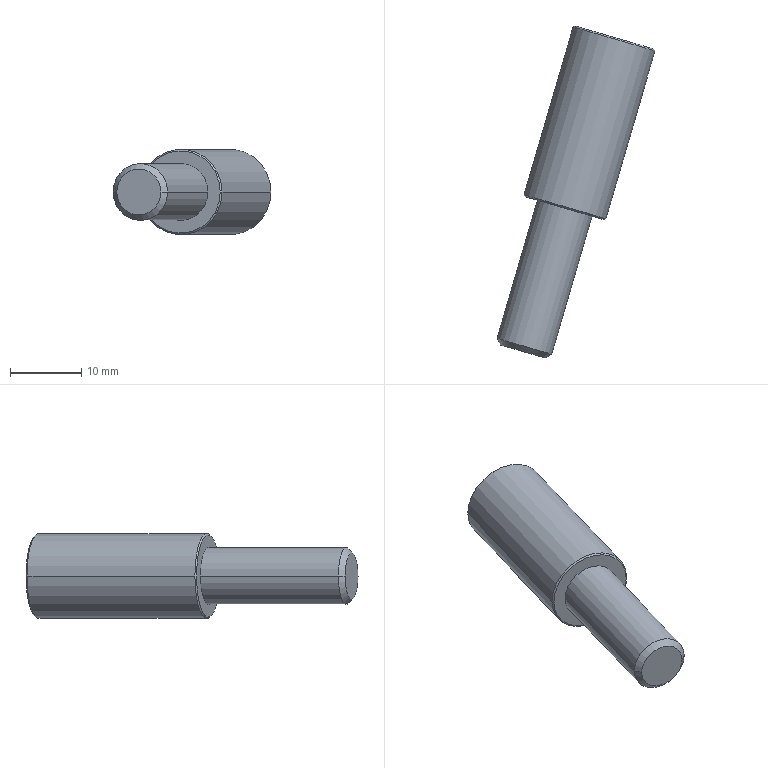Part | SolidWorks | features BaseBody 1 | 1 solid | 31 faces | box 22.207 x 46.689 x 12 mm | volume 3091 mm3 | plane 15 | cone 10 | cylinder 6 | commonest cylinder face diameters 6.647 x2 8 x2 12 x2
STEP:
#1=CARTESIAN_POINT('',(21.689,446.862,-1.629));
#2=VERTEX_POINT('',#1);
#3=CARTESIAN_POINT('',(10.169,450.221,-1.629));
#4=VERTEX_POINT('',#3);
#5=CARTESIAN_POINT('',(15.929,448.541,-1.629));
#6=DIRECTION('',(-0.28,-0.96,0.));
#7=DIRECTION('',(0.96,-0.28,0.));
#8=AXIS2_PLACEMENT_3D('',#5,#6,#7);
#9=CIRCLE('',#8,6.);
#10=EDGE_CURVE('',#2,#4,#9,.T.);
#11=ORIENTED_EDGE('',*,*,#10,.T.);
#12=CARTESIAN_POINT('',(3.282,426.605,-1.629));
#13=VERTEX_POINT('',#12);
#14=CARTESIAN_POINT('',(6.726,438.413,-1.629));
#15=DIRECTION('',(-0.28,-0.96,0.));
#16=VECTOR('',#15,1000.);
#17=LINE('',#14,#16);
#18=EDGE_CURVE('',#4,#13,#17,.T.);
#19=ORIENTED_EDGE('',*,*,#18,.T.);
#20=CARTESIAN_POINT('',(14.802,423.245,-1.629));
#21=VERTEX_POINT('',#20);
#22=CARTESIAN_POINT('',(9.042,424.925,-1.629));
#23=DIRECTION('',(0.28,0.96,0.));
#24=DIRECTION('',(0.96,-0.28,0.));
#25=AXIS2_PLACEMENT_3D('',#22,#23,#24);
#26=CIRCLE('',#25,6.);
#27=EDGE_CURVE('',#13,#21,#26,.T.);
#28=ORIENTED_EDGE('',*,*,#27,.T.);
#29=CARTESIAN_POINT('',(18.246,435.053,-1.629));
#30=DIRECTION('',(-0.28,-0.96,0.));
#31=VECTOR('',#30,1000.);
#32=LINE('',#29,#31);
#33=EDGE_CURVE('',#2,#21,#32,.T.);
#34=ORIENTED_EDGE('',*,*,#33,.F.);
#35=EDGE_LOOP('',(#11,#19,#28,#34));
#36=FACE_OUTER_BOUND('',#35,.T.);
#37=CARTESIAN_POINT('',(12.486,436.733,-1.629));
#38=DIRECTION('',(-0.28,-0.96,0.));
#39=DIRECTION('',(0.96,-0.28,0.));
#40=AXIS2_PLACEMENT_3D('',#37,#38,#39);
#41=CYLINDRICAL_SURFACE('',#40,6.);
#42=ADVANCED_FACE('',(#36),#41,.T.);
#43=CARTESIAN_POINT('',(3.418,426.357,-1.629));
#44=VERTEX_POINT('',#43);
#45=CARTESIAN_POINT('',(14.554,423.109,-1.629));
#46=VERTEX_POINT('',#45);
#47=CARTESIAN_POINT('',(8.986,424.733,-1.629));
#48=DIRECTION('',(0.28,0.96,0.));
#49=DIRECTION('',(-0.96,0.28,0.));
#50=AXIS2_PLACEMENT_3D('',#47,#48,#49);
#51=CIRCLE('',#50,5.8);
#52=EDGE_CURVE('',#44,#46,#51,.T.);
#53=ORIENTED_EDGE('',*,*,#52,.T.);
#54=CARTESIAN_POINT('',(14.802,423.245,-1.629));
#55=DIRECTION('',(0.8768,0.4809,0.));
#56=VECTOR('',#55,1000.);
#57=LINE('',#54,#56);
#58=EDGE_CURVE('',#46,#21,#57,.T.);
#59=ORIENTED_EDGE('',*,*,#58,.T.);
#60=ORIENTED_EDGE('',*,*,#27,.F.);
#61=CARTESIAN_POINT('',(3.282,426.605,-1.629));
#62=DIRECTION('',(-0.4809,0.8768,0.));
#63=VECTOR('',#62,1000.);
#64=LINE('',#61,#63);
#65=EDGE_CURVE('',#44,#13,#64,.T.);
#66=ORIENTED_EDGE('',*,*,#65,.F.);
#67=EDGE_LOOP('',(#53,#59,#60,#66));
#68=FACE_OUTER_BOUND('',#67,.T.);
#69=CARTESIAN_POINT('',(9.042,424.925,-1.629));
#70=DIRECTION('',(0.28,0.96,0.));
#71=DIRECTION('',(-0.96,0.28,0.));
#72=AXIS2_PLACEMENT_3D('',#69,#70,#71);
#73=CONICAL_SURFACE('',#72,6.,0.7854);
#74=ADVANCED_FACE('',(#68),#73,.T.);
#75=CARTESIAN_POINT('',(21.553,447.11,-1.629));
#76=VERTEX_POINT('',#75);
#77=CARTESIAN_POINT('',(10.417,450.357,-1.629));
#78=VERTEX_POINT('',#77);
#79=CARTESIAN_POINT('',(15.985,448.733,-1.629));
#80=DIRECTION('',(-0.28,-0.96,0.));
#81=DIRECTION('',(0.96,-0.28,0.));
#82=AXIS2_PLACEMENT_3D('',#79,#80,#81);
#83=CIRCLE('',#82,5.8);
#84=EDGE_CURVE('',#76,#78,#83,.T.);
#85=ORIENTED_EDGE('',*,*,#84,.T.);
#86=CARTESIAN_POINT('',(10.169,450.221,-1.629));
#87=DIRECTION('',(-0.8768,-0.4809,0.));
#88=VECTOR('',#87,1000.);
#89=LINE('',#86,#88);
#90=EDGE_CURVE('',#78,#4,#89,.T.);
#91=ORIENTED_EDGE('',*,*,#90,.T.);
#92=ORIENTED_EDGE('',*,*,#10,.F.);
#93=CARTESIAN_POINT('',(21.689,446.862,-1.629));
#94=DIRECTION('',(0.4809,-0.8768,0.));
#95=VECTOR('',#94,1000.);
#96=LINE('',#93,#95);
#97=EDGE_CURVE('',#76,#2,#96,.T.);
#98=ORIENTED_EDGE('',*,*,#97,.F.);
#99=EDGE_LOOP('',(#85,#91,#92,#98));
#100=FACE_OUTER_BOUND('',#99,.T.);
#101=CARTESIAN_POINT('',(15.929,448.541,-1.629));
#102=DIRECTION('',(-0.28,-0.96,0.));
#103=DIRECTION('',(0.96,-0.28,0.));
#104=AXIS2_PLACEMENT_3D('',#101,#102,#103);
#105=CONICAL_SURFACE('',#104,6.,0.7854);
#106=ADVANCED_FACE('',(#100),#105,.T.);
#107=CARTESIAN_POINT('',(5.146,425.853,-1.629));
#108=VERTEX_POINT('',#107);
#109=CARTESIAN_POINT('',(12.826,423.613,-1.629));
#110=VERTEX_POINT('',#109);
#111=CARTESIAN_POINT('',(8.986,424.733,-1.629));
#112=DIRECTION('',(0.28,0.96,0.));
#113=DIRECTION('',(0.96,-0.28,0.));
#114=AXIS2_PLACEMENT_3D('',#111,#112,#113);
#115=CIRCLE('',#114,4.);
#116=EDGE_CURVE('',#108,#110,#115,.T.);
#117=ORIENTED_EDGE('',*,*,#116,.F.);
#118=CARTESIAN_POINT('',(-0.5181,406.429,-1.629));
#119=VERTEX_POINT('',#118);
#120=CARTESIAN_POINT('',(2.314,416.141,-1.629));
#121=DIRECTION('',(-0.28,-0.96,0.));
#122=VECTOR('',#121,1000.);
#123=LINE('',#120,#122);
#124=EDGE_CURVE('',#108,#119,#123,.T.);
#125=ORIENTED_EDGE('',*,*,#124,.T.);
#126=CARTESIAN_POINT('',(7.162,404.189,-1.629));
#127=VERTEX_POINT('',#126);
#128=CARTESIAN_POINT('',(3.322,405.309,-1.629));
#129=DIRECTION('',(0.28,0.96,0.));
#130=DIRECTION('',(0.96,-0.28,0.));
#131=AXIS2_PLACEMENT_3D('',#128,#129,#130);
#132=CIRCLE('',#131,4.);
#133=EDGE_CURVE('',#119,#127,#132,.T.);
#134=ORIENTED_EDGE('',*,*,#133,.T.);
#135=CARTESIAN_POINT('',(9.994,413.901,-1.629));
#136=DIRECTION('',(-0.28,-0.96,0.));
#137=VECTOR('',#136,1000.);
#138=LINE('',#135,#137);
#139=EDGE_CURVE('',#110,#127,#138,.T.);
#140=ORIENTED_EDGE('',*,*,#139,.F.);
#141=EDGE_LOOP('',(#117,#125,#134,#140));
#142=FACE_OUTER_BOUND('',#141,.T.);
#143=CARTESIAN_POINT('',(6.154,415.021,-1.629));
#144=DIRECTION('',(-0.28,-0.96,0.));
#145=DIRECTION('',(0.96,-0.28,0.));
#146=AXIS2_PLACEMENT_3D('',#143,#144,#145);
#147=CYLINDRICAL_SURFACE('',#146,4.);
#148=ADVANCED_FACE('',(#142),#147,.T.);
#149=CARTESIAN_POINT('',(0.003527,405.478,-1.629));
#150=VERTEX_POINT('',#149);
#151=CARTESIAN_POINT('',(6.211,403.668,-1.629));
#152=VERTEX_POINT('',#151);
#153=CARTESIAN_POINT('',(3.107,404.573,-1.629));
#154=DIRECTION('',(0.28,0.96,0.));
#155=DIRECTION('',(-0.96,0.28,0.));
#156=AXIS2_PLACEMENT_3D('',#153,#154,#155);
#157=CIRCLE('',#156,3.233);
#158=EDGE_CURVE('',#150,#152,#157,.T.);
#159=ORIENTED_EDGE('',*,*,#158,.T.);
#160=CARTESIAN_POINT('',(7.162,404.189,-1.629));
#161=DIRECTION('',(0.8768,0.4809,0.));
#162=VECTOR('',#161,1000.);
#163=LINE('',#160,#162);
#164=EDGE_CURVE('',#152,#127,#163,.T.);
#165=ORIENTED_EDGE('',*,*,#164,.T.);
#166=ORIENTED_EDGE('',*,*,#133,.F.);
#167=CARTESIAN_POINT('',(-0.5181,406.429,-1.629));
#168=DIRECTION('',(-0.4809,0.8768,0.));
#169=VECTOR('',#168,1000.);
#170=LINE('',#167,#169);
#171=EDGE_CURVE('',#150,#119,#170,.T.);
#172=ORIENTED_EDGE('',*,*,#171,.F.);
#173=EDGE_LOOP('',(#159,#165,#166,#172));
#174=FACE_OUTER_BOUND('',#173,.T.);
#175=CARTESIAN_POINT('',(3.322,405.309,-1.629));
#176=DIRECTION('',(0.28,0.96,0.));
#177=DIRECTION('',(-0.96,0.28,0.));
#178=AXIS2_PLACEMENT_3D('',#175,#176,#177);
#179=CONICAL_SURFACE('',#178,4.,0.7854);
#180=ADVANCED_FACE('',(#174),#179,.T.);
#181=CARTESIAN_POINT('',(18.146,444.273,-1.629));
#182=VERTEX_POINT('',#181);
#183=CARTESIAN_POINT('',(11.765,446.134,-1.629));
#184=VERTEX_POINT('',#183);
#185=CARTESIAN_POINT('',(14.956,445.204,-1.629));
#186=DIRECTION('',(0.28,0.96,0.));
#187=DIRECTION('',(0.,0.,1.));
#188=AXIS2_PLACEMENT_3D('',#185,#186,#187);
#189=CIRCLE('',#188,3.324);
#190=EDGE_CURVE('',#182,#184,#189,.T.);
#191=ORIENTED_EDGE('',*,*,#190,.F.);
#192=CARTESIAN_POINT('',(18.985,444.733,-1.629));
#193=VERTEX_POINT('',#192);
#194=CARTESIAN_POINT('',(18.985,444.733,-1.629));
#195=DIRECTION('',(0.8768,0.4809,0.));
#196=VECTOR('',#195,1000.);
#197=LINE('',#194,#196);
#198=EDGE_CURVE('',#182,#193,#197,.T.);
#199=ORIENTED_EDGE('',*,*,#198,.T.);
#200=CARTESIAN_POINT('',(17.065,445.293,-5.093));
#201=VERTEX_POINT('',#200);
#202=CARTESIAN_POINT('',(15.145,445.853,-1.629));
#203=DIRECTION('',(0.28,0.96,0.));
#204=DIRECTION('',(-0.96,0.28,0.));
#205=AXIS2_PLACEMENT_3D('',#202,#203,#204);
#206=CIRCLE('',#205,4.);
#207=EDGE_CURVE('',#193,#201,#206,.T.);
#208=ORIENTED_EDGE('',*,*,#207,.T.);
#209=CARTESIAN_POINT('',(13.225,446.413,-5.093));
#210=VERTEX_POINT('',#209);
#211=CARTESIAN_POINT('',(15.145,445.853,-1.629));
#212=DIRECTION('',(0.28,0.96,0.));
#213=DIRECTION('',(-0.96,0.28,0.));
#214=AXIS2_PLACEMENT_3D('',#211,#212,#213);
#215=CIRCLE('',#214,4.);
#216=EDGE_CURVE('',#201,#210,#215,.T.);
#217=ORIENTED_EDGE('',*,*,#216,.T.);
#218=CARTESIAN_POINT('',(11.305,446.973,-1.629));
#219=VERTEX_POINT('',#218);
#220=CARTESIAN_POINT('',(15.145,445.853,-1.629));
#221=DIRECTION('',(0.28,0.96,0.));
#222=DIRECTION('',(-0.96,0.28,0.));
#223=AXIS2_PLACEMENT_3D('',#220,#221,#222);
#224=CIRCLE('',#223,4.);
#225=EDGE_CURVE('',#210,#219,#224,.T.);
#226=ORIENTED_EDGE('',*,*,#225,.T.);
#227=CARTESIAN_POINT('',(11.305,446.973,-1.629));
#228=DIRECTION('',(-0.4809,0.8768,0.));
#229=VECTOR('',#228,1000.);
#230=LINE('',#227,#229);
#231=EDGE_CURVE('',#184,#219,#230,.T.);
#232=ORIENTED_EDGE('',*,*,#231,.F.);
#233=EDGE_LOOP('',(#191,#199,#208,#217,#226,#232));
#234=FACE_OUTER_BOUND('',#233,.T.);
#235=CARTESIAN_POINT('',(15.145,445.853,-1.629));
#236=DIRECTION('',(0.28,0.96,0.));
#237=DIRECTION('',(-0.96,0.28,0.));
#238=AXIS2_PLACEMENT_3D('',#235,#236,#237);
#239=CONICAL_SURFACE('',#238,4.,0.7854);
#240=ADVANCED_FACE('',(#234),#239,.F.);
#241=ORIENTED_EDGE('',*,*,#190,.T.);
#242=CARTESIAN_POINT('',(7.195,430.463,-1.629));
#243=VERTEX_POINT('',#242);
#244=CARTESIAN_POINT('',(9.48,438.299,-1.629));
#245=DIRECTION('',(-0.28,-0.96,0.));
#246=VECTOR('',#245,1000.);
#247=LINE('',#244,#246);
#248=EDGE_CURVE('',#184,#243,#247,.T.);
#249=ORIENTED_EDGE('',*,*,#248,.T.);
#250=CARTESIAN_POINT('',(13.577,428.603,-1.629));
#251=VERTEX_POINT('',#250);
#252=CARTESIAN_POINT('',(10.386,429.533,-1.629));
#253=DIRECTION('',(0.28,0.96,0.));
#254=DIRECTION('',(0.96,-0.28,0.));
#255=AXIS2_PLACEMENT_3D('',#252,#253,#254);
#256=CIRCLE('',#255,3.324);
#257=EDGE_CURVE('',#251,#243,#256,.T.);
#258=ORIENTED_EDGE('',*,*,#257,.F.);
#259=CARTESIAN_POINT('',(15.862,436.438,-1.629));
#260=DIRECTION('',(-0.28,-0.96,0.));
#261=VECTOR('',#260,1000.);
#262=LINE('',#259,#261);
#263=EDGE_CURVE('',#182,#251,#262,.T.);
#264=ORIENTED_EDGE('',*,*,#263,.F.);
#265=EDGE_LOOP('',(#241,#249,#258,#264));
#266=FACE_OUTER_BOUND('',#265,.T.);
#267=CARTESIAN_POINT('',(12.671,437.368,-1.629));
#268=DIRECTION('',(-0.28,-0.96,0.));
#269=DIRECTION('',(0.96,-0.28,0.));
#270=AXIS2_PLACEMENT_3D('',#267,#268,#269);
#271=CYLINDRICAL_SURFACE('',#270,3.324);
#272=ADVANCED_FACE('',(#266),#271,.F.);
#273=CARTESIAN_POINT('',(9.849,427.691,-1.629));
#274=VERTEX_POINT('',#273);
#275=CARTESIAN_POINT('',(7.195,430.463,-1.629));
#276=DIRECTION('',(-0.6914,0.7225,0.));
#277=VECTOR('',#276,1000.);
#278=LINE('',#275,#277);
#279=EDGE_CURVE('',#274,#243,#278,.T.);
#280=ORIENTED_EDGE('',*,*,#279,.F.);
#281=CARTESIAN_POINT('',(13.577,428.603,-1.629));
#282=DIRECTION('',(0.9714,0.2376,0.));
#283=VECTOR('',#282,1000.);
#284=LINE('',#281,#283);
#285=EDGE_CURVE('',#274,#251,#284,.T.);
#286=ORIENTED_EDGE('',*,*,#285,.T.);
#287=ORIENTED_EDGE('',*,*,#257,.T.);
#288=EDGE_LOOP('',(#280,#286,#287));
#289=FACE_OUTER_BOUND('',#288,.T.);
#290=CARTESIAN_POINT('',(10.386,429.533,-1.629));
#291=DIRECTION('',(0.28,0.96,0.));
#292=DIRECTION('',(-0.96,0.28,0.));
#293=AXIS2_PLACEMENT_3D('',#290,#291,#292);
#294=CONICAL_SURFACE('',#293,3.324,1.047);
#295=ADVANCED_FACE('',(#289),#294,.F.);
#296=ORIENTED_EDGE('',*,*,#18,.F.);
#297=CARTESIAN_POINT('',(15.929,448.541,-1.629));
#298=DIRECTION('',(-0.28,-0.96,0.));
#299=DIRECTION('',(0.96,-0.28,0.));
#300=AXIS2_PLACEMENT_3D('',#297,#298,#299);
#301=CIRCLE('',#300,6.);
#302=EDGE_CURVE('',#4,#2,#301,.T.);
#303=ORIENTED_EDGE('',*,*,#302,.T.);
#304=ORIENTED_EDGE('',*,*,#33,.T.);
#305=CARTESIAN_POINT('',(9.042,424.925,-1.629));
#306=DIRECTION('',(0.28,0.96,0.));
#307=DIRECTION('',(0.96,-0.28,0.));
#308=AXIS2_PLACEMENT_3D('',#305,#306,#307);
#309=CIRCLE('',#308,6.);
#310=EDGE_CURVE('',#21,#13,#309,.T.);
#311=ORIENTED_EDGE('',*,*,#310,.T.);
#312=EDGE_LOOP('',(#296,#303,#304,#311));
#313=FACE_OUTER_BOUND('',#312,.T.);
#314=CARTESIAN_POINT('',(12.486,436.733,-1.629));
#315=DIRECTION('',(-0.28,-0.96,0.));
#316=DIRECTION('',(0.96,-0.28,0.));
#317=AXIS2_PLACEMENT_3D('',#314,#315,#316);
#318=CYLINDRICAL_SURFACE('',#317,6.);
#319=ADVANCED_FACE('',(#313),#318,.T.);
#320=ORIENTED_EDGE('',*,*,#58,.F.);
#321=CARTESIAN_POINT('',(8.986,424.733,-1.629));
#322=DIRECTION('',(0.28,0.96,0.));
#323=DIRECTION('',(-0.96,0.28,0.));
#324=AXIS2_PLACEMENT_3D('',#321,#322,#323);
#325=CIRCLE('',#324,5.8);
#326=EDGE_CURVE('',#46,#44,#325,.T.);
#327=ORIENTED_EDGE('',*,*,#326,.T.);
#328=ORIENTED_EDGE('',*,*,#65,.T.);
#329=ORIENTED_EDGE('',*,*,#310,.F.);
#330=EDGE_LOOP('',(#320,#327,#328,#329));
#331=FACE_OUTER_BOUND('',#330,.T.);
#332=CARTESIAN_POINT('',(9.042,424.925,-1.629));
#333=DIRECTION('',(0.28,0.96,0.));
#334=DIRECTION('',(-0.96,0.28,0.));
#335=AXIS2_PLACEMENT_3D('',#332,#333,#334);
#336=CONICAL_SURFACE('',#335,6.,0.7854);
#337=ADVANCED_FACE('',(#331),#336,.T.);
#338=ORIENTED_EDGE('',*,*,#90,.F.);
#339=CARTESIAN_POINT('',(15.985,448.733,-1.629));
#340=DIRECTION('',(-0.28,-0.96,0.));
#341=DIRECTION('',(0.96,-0.28,0.));
#342=AXIS2_PLACEMENT_3D('',#339,#340,#341);
#343=CIRCLE('',#342,5.8);
#344=EDGE_CURVE('',#78,#76,#343,.T.);
#345=ORIENTED_EDGE('',*,*,#344,.T.);
#346=ORIENTED_EDGE('',*,*,#97,.T.);
#347=ORIENTED_EDGE('',*,*,#302,.F.);
#348=EDGE_LOOP('',(#338,#345,#346,#347));
#349=FACE_OUTER_BOUND('',#348,.T.);
#350=CARTESIAN_POINT('',(15.929,448.541,-1.629));
#351=DIRECTION('',(-0.28,-0.96,0.));
#352=DIRECTION('',(0.96,-0.28,0.));
#353=AXIS2_PLACEMENT_3D('',#350,#351,#352);
#354=CONICAL_SURFACE('',#353,6.,0.7854);
#355=ADVANCED_FACE('',(#349),#354,.T.);
#356=ORIENTED_EDGE('',*,*,#52,.F.);
#357=ORIENTED_EDGE('',*,*,#326,.F.);
#358=EDGE_LOOP('',(#356,#357));
#359=FACE_OUTER_BOUND('',#358,.T.);
#360=CARTESIAN_POINT('',(8.986,424.733,-1.629));
#361=DIRECTION('',(0.28,0.96,0.));
#362=DIRECTION('',(0.96,-0.28,0.));
#363=AXIS2_PLACEMENT_3D('',#360,#361,#362);
#364=CIRCLE('',#363,4.);
#365=EDGE_CURVE('',#110,#108,#364,.T.);
#366=ORIENTED_EDGE('',*,*,#365,.T.);
#367=ORIENTED_EDGE('',*,*,#116,.T.);
#368=EDGE_LOOP('',(#366,#367));
#369=FACE_BOUND('',#368,.T.);
#370=CARTESIAN_POINT('',(8.986,424.733,1.271));
#371=DIRECTION('',(-0.28,-0.96,0.));
#372=DIRECTION('',(0.96,-0.28,0.));
#373=AXIS2_PLACEMENT_3D('',#370,#371,#372);
#374=PLANE('',#373);
#375=ADVANCED_FACE('',(#359,#369),#374,.T.);
#376=CARTESIAN_POINT('',(12.145,449.853,-3.938));
#377=VERTEX_POINT('',#376);
#378=CARTESIAN_POINT('',(15.985,448.733,-6.248));
#379=VERTEX_POINT('',#378);
#380=CARTESIAN_POINT('',(12.145,449.853,-3.938));
#381=DIRECTION('',(0.8314,-0.2424,-0.5));
#382=VECTOR('',#381,1000.);
#383=LINE('',#380,#382);
#384=EDGE_CURVE('',#377,#379,#383,.T.);
#385=ORIENTED_EDGE('',*,*,#384,.T.);
#386=CARTESIAN_POINT('',(19.825,447.613,-3.938));
#387=VERTEX_POINT('',#386);
#388=CARTESIAN_POINT('',(15.985,448.733,-6.248));
#389=DIRECTION('',(0.8314,-0.2424,0.5));
#390=VECTOR('',#389,1000.);
#391=LINE('',#388,#390);
#392=EDGE_CURVE('',#379,#387,#391,.T.);
#393=ORIENTED_EDGE('',*,*,#392,.T.);
#394=CARTESIAN_POINT('',(19.825,447.613,0.6805));
#395=VERTEX_POINT('',#394);
#396=CARTESIAN_POINT('',(19.825,447.613,1.271));
#397=DIRECTION('',(0.,0.,1.));
#398=VECTOR('',#397,1000.);
#399=LINE('',#396,#398);
#400=EDGE_CURVE('',#387,#395,#399,.T.);
#401=ORIENTED_EDGE('',*,*,#400,.T.);
#402=CARTESIAN_POINT('',(15.985,448.733,2.99));
#403=VERTEX_POINT('',#402);
#404=CARTESIAN_POINT('',(19.825,447.613,0.6805));
#405=DIRECTION('',(-0.8314,0.2424,0.5));
#406=VECTOR('',#405,1000.);
#407=LINE('',#404,#406);
#408=EDGE_CURVE('',#395,#403,#407,.T.);
#409=ORIENTED_EDGE('',*,*,#408,.T.);
#410=CARTESIAN_POINT('',(12.145,449.853,0.6805));
#411=VERTEX_POINT('',#410);
#412=CARTESIAN_POINT('',(15.985,448.733,2.99));
#413=DIRECTION('',(-0.8314,0.2424,-0.5));
#414=VECTOR('',#413,1000.);
#415=LINE('',#412,#414);
#416=EDGE_CURVE('',#403,#411,#415,.T.);
#417=ORIENTED_EDGE('',*,*,#416,.T.);
#418=CARTESIAN_POINT('',(12.145,449.853,1.271));
#419=DIRECTION('',(0.,0.,-1.));
#420=VECTOR('',#419,1000.);
#421=LINE('',#418,#420);
#422=EDGE_CURVE('',#411,#377,#421,.T.);
#423=ORIENTED_EDGE('',*,*,#422,.T.);
#424=EDGE_LOOP('',(#385,#393,#401,#409,#417,#423));
#425=FACE_BOUND('',#424,.T.);
#426=ORIENTED_EDGE('',*,*,#84,.F.);
#427=ORIENTED_EDGE('',*,*,#344,.F.);
#428=EDGE_LOOP('',(#426,#427));
#429=FACE_OUTER_BOUND('',#428,.T.);
#430=CARTESIAN_POINT('',(15.985,448.733,1.271));
#431=DIRECTION('',(0.28,0.96,0.));
#432=DIRECTION('',(-0.96,0.28,0.));
#433=AXIS2_PLACEMENT_3D('',#430,#431,#432);
#434=PLANE('',#433);
#435=ADVANCED_FACE('',(#425,#429),#434,.T.);
#436=ORIENTED_EDGE('',*,*,#124,.F.);
#437=ORIENTED_EDGE('',*,*,#365,.F.);
#438=ORIENTED_EDGE('',*,*,#139,.T.);
#439=CARTESIAN_POINT('',(3.322,405.309,-1.629));
#440=DIRECTION('',(0.28,0.96,0.));
#441=DIRECTION('',(0.96,-0.28,0.));
#442=AXIS2_PLACEMENT_3D('',#439,#440,#441);
#443=CIRCLE('',#442,4.);
#444=EDGE_CURVE('',#127,#119,#443,.T.);
#445=ORIENTED_EDGE('',*,*,#444,.T.);
#446=EDGE_LOOP('',(#436,#437,#438,#445));
#447=FACE_OUTER_BOUND('',#446,.T.);
#448=CARTESIAN_POINT('',(6.154,415.021,-1.629));
#449=DIRECTION('',(-0.28,-0.96,0.));
#450=DIRECTION('',(0.96,-0.28,0.));
#451=AXIS2_PLACEMENT_3D('',#448,#449,#450);
#452=CYLINDRICAL_SURFACE('',#451,4.);
#453=ADVANCED_FACE('',(#447),#452,.T.);
#454=ORIENTED_EDGE('',*,*,#392,.F.);
#455=CARTESIAN_POINT('',(15.145,445.853,-6.248));
#456=VERTEX_POINT('',#455);
#457=CARTESIAN_POINT('',(15.145,445.853,-6.248));
#458=DIRECTION('',(0.28,0.96,0.));
#459=VECTOR('',#458,1000.);
#460=LINE('',#457,#459);
#461=EDGE_CURVE('',#456,#379,#460,.T.);
#462=ORIENTED_EDGE('',*,*,#461,.F.);
#463=CARTESIAN_POINT('',(17.065,445.293,-5.093));
#464=DIRECTION('',(-0.8314,0.2424,-0.5));
#465=VECTOR('',#464,1000.);
#466=LINE('',#463,#465);
#467=EDGE_CURVE('',#201,#456,#466,.T.);
#468=ORIENTED_EDGE('',*,*,#467,.F.);
#469=CARTESIAN_POINT('',(18.985,444.733,-3.938));
#470=VERTEX_POINT('',#469);
#471=CARTESIAN_POINT('',(18.985,444.733,-3.938));
#472=DIRECTION('',(-0.8314,0.2424,-0.5));
#473=VECTOR('',#472,1000.);
#474=LINE('',#471,#473);
#475=EDGE_CURVE('',#470,#201,#474,.T.);
#476=ORIENTED_EDGE('',*,*,#475,.F.);
#477=CARTESIAN_POINT('',(19.825,447.613,-3.938));
#478=DIRECTION('',(-0.28,-0.96,0.));
#479=VECTOR('',#478,1000.);
#480=LINE('',#477,#479);
#481=EDGE_CURVE('',#387,#470,#480,.T.);
#482=ORIENTED_EDGE('',*,*,#481,.F.);
#483=EDGE_LOOP('',(#454,#462,#468,#476,#482));
#484=FACE_OUTER_BOUND('',#483,.T.);
#485=CARTESIAN_POINT('',(19.825,447.613,-3.938));
#486=DIRECTION('',(0.48,-0.14,-0.866));
#487=DIRECTION('',(-0.8746,0.,-0.4848));
#488=AXIS2_PLACEMENT_3D('',#485,#486,#487);
#489=PLANE('',#488);
#490=ADVANCED_FACE('',(#484),#489,.F.);
#491=ORIENTED_EDGE('',*,*,#384,.F.);
#492=CARTESIAN_POINT('',(11.305,446.973,-3.938));
#493=VERTEX_POINT('',#492);
#494=CARTESIAN_POINT('',(11.305,446.973,-3.938));
#495=DIRECTION('',(0.28,0.96,0.));
#496=VECTOR('',#495,1000.);
#497=LINE('',#494,#496);
#498=EDGE_CURVE('',#493,#377,#497,.T.);
#499=ORIENTED_EDGE('',*,*,#498,.F.);
#500=CARTESIAN_POINT('',(13.225,446.413,-5.093));
#501=DIRECTION('',(-0.8314,0.2424,0.5));
#502=VECTOR('',#501,1000.);
#503=LINE('',#500,#502);
#504=EDGE_CURVE('',#210,#493,#503,.T.);
#505=ORIENTED_EDGE('',*,*,#504,.F.);
#506=CARTESIAN_POINT('',(15.145,445.853,-6.248));
#507=DIRECTION('',(-0.8314,0.2424,0.5));
#508=VECTOR('',#507,1000.);
#509=LINE('',#506,#508);
#510=EDGE_CURVE('',#456,#210,#509,.T.);
#511=ORIENTED_EDGE('',*,*,#510,.F.);
#512=ORIENTED_EDGE('',*,*,#461,.T.);
#513=EDGE_LOOP('',(#491,#499,#505,#511,#512));
#514=FACE_OUTER_BOUND('',#513,.T.);
#515=CARTESIAN_POINT('',(15.985,448.733,-6.248));
#516=DIRECTION('',(-0.48,0.14,-0.866));
#517=DIRECTION('',(-0.8746,0.,0.4848));
#518=AXIS2_PLACEMENT_3D('',#515,#516,#517);
#519=PLANE('',#518);
#520=ADVANCED_FACE('',(#514),#519,.F.);
#521=ORIENTED_EDGE('',*,*,#422,.F.);
#522=CARTESIAN_POINT('',(11.305,446.973,0.6805));
#523=VERTEX_POINT('',#522);
#524=CARTESIAN_POINT('',(12.145,449.853,0.6805));
#525=DIRECTION('',(0.28,0.96,0.));
#526=VECTOR('',#525,1000.);
#527=LINE('',#524,#526);
#528=EDGE_CURVE('',#523,#411,#527,.T.);
#529=ORIENTED_EDGE('',*,*,#528,.F.);
#530=CARTESIAN_POINT('',(11.305,446.973,-3.938));
#531=DIRECTION('',(0.,0.,1.));
#532=VECTOR('',#531,1000.);
#533=LINE('',#530,#532);
#534=EDGE_CURVE('',#219,#523,#533,.T.);
#535=ORIENTED_EDGE('',*,*,#534,.F.);
#536=CARTESIAN_POINT('',(11.305,446.973,-3.938));
#537=DIRECTION('',(0.,0.,1.));
#538=VECTOR('',#537,1000.);
#539=LINE('',#536,#538);
#540=EDGE_CURVE('',#493,#219,#539,.T.);
#541=ORIENTED_EDGE('',*,*,#540,.F.);
#542=ORIENTED_EDGE('',*,*,#498,.T.);
#543=EDGE_LOOP('',(#521,#529,#535,#541,#542));
#544=FACE_OUTER_BOUND('',#543,.T.);
#545=CARTESIAN_POINT('',(12.145,449.853,-3.938));
#546=DIRECTION('',(-0.96,0.28,0.));
#547=DIRECTION('',(-0.28,-0.96,0.));
#548=AXIS2_PLACEMENT_3D('',#545,#546,#547);
#549=PLANE('',#548);
#550=ADVANCED_FACE('',(#544),#549,.F.);
#551=ORIENTED_EDGE('',*,*,#416,.F.);
#552=CARTESIAN_POINT('',(15.145,445.853,2.99));
#553=VERTEX_POINT('',#552);
#554=CARTESIAN_POINT('',(15.145,445.853,2.99));
#555=DIRECTION('',(0.28,0.96,0.));
#556=VECTOR('',#555,1000.);
#557=LINE('',#554,#556);
#558=EDGE_CURVE('',#553,#403,#557,.T.);
#559=ORIENTED_EDGE('',*,*,#558,.F.);
#560=CARTESIAN_POINT('',(13.225,446.413,1.835));
#561=VERTEX_POINT('',#560);
#562=CARTESIAN_POINT('',(13.225,446.413,1.835));
#563=DIRECTION('',(0.8314,-0.2424,0.5));
#564=VECTOR('',#563,1000.);
#565=LINE('',#562,#564);
#566=EDGE_CURVE('',#561,#553,#565,.T.);
#567=ORIENTED_EDGE('',*,*,#566,.F.);
#568=CARTESIAN_POINT('',(11.305,446.973,0.6805));
#569=DIRECTION('',(0.8314,-0.2424,0.5));
#570=VECTOR('',#569,1000.);
#571=LINE('',#568,#570);
#572=EDGE_CURVE('',#523,#561,#571,.T.);
#573=ORIENTED_EDGE('',*,*,#572,.F.);
#574=ORIENTED_EDGE('',*,*,#528,.T.);
#575=EDGE_LOOP('',(#551,#559,#567,#573,#574));
#576=FACE_OUTER_BOUND('',#575,.T.);
#577=CARTESIAN_POINT('',(12.145,449.853,0.6805));
#578=DIRECTION('',(-0.48,0.14,0.866));
#579=DIRECTION('',(0.8746,0.,0.4848));
#580=AXIS2_PLACEMENT_3D('',#577,#578,#579);
#581=PLANE('',#580);
#582=ADVANCED_FACE('',(#576),#581,.F.);
#583=ORIENTED_EDGE('',*,*,#408,.F.);
#584=CARTESIAN_POINT('',(18.985,444.733,0.6805));
#585=VERTEX_POINT('',#584);
#586=CARTESIAN_POINT('',(18.985,444.733,0.6805));
#587=DIRECTION('',(0.28,0.96,0.));
#588=VECTOR('',#587,1000.);
#589=LINE('',#586,#588);
#590=EDGE_CURVE('',#585,#395,#589,.T.);
#591=ORIENTED_EDGE('',*,*,#590,.F.);
#592=CARTESIAN_POINT('',(17.065,445.293,1.835));
#593=VERTEX_POINT('',#592);
#594=CARTESIAN_POINT('',(17.065,445.293,1.835));
#595=DIRECTION('',(0.8314,-0.2424,-0.5));
#596=VECTOR('',#595,1000.);
#597=LINE('',#594,#596);
#598=EDGE_CURVE('',#593,#585,#597,.T.);
#599=ORIENTED_EDGE('',*,*,#598,.F.);
#600=CARTESIAN_POINT('',(15.145,445.853,2.99));
#601=DIRECTION('',(0.8314,-0.2424,-0.5));
#602=VECTOR('',#601,1000.);
#603=LINE('',#600,#602);
#604=EDGE_CURVE('',#553,#593,#603,.T.);
#605=ORIENTED_EDGE('',*,*,#604,.F.);
#606=ORIENTED_EDGE('',*,*,#558,.T.);
#607=EDGE_LOOP('',(#583,#591,#599,#605,#606));
#608=FACE_OUTER_BOUND('',#607,.T.);
#609=CARTESIAN_POINT('',(15.985,448.733,2.99));
#610=DIRECTION('',(0.48,-0.14,0.866));
#611=DIRECTION('',(0.8746,0.,-0.4848));
#612=AXIS2_PLACEMENT_3D('',#609,#610,#611);
#613=PLANE('',#612);
#614=ADVANCED_FACE('',(#608),#613,.F.);
#615=ORIENTED_EDGE('',*,*,#400,.F.);
#616=ORIENTED_EDGE('',*,*,#481,.T.);
#617=CARTESIAN_POINT('',(18.985,444.733,0.6805));
#618=DIRECTION('',(0.,0.,-1.));
#619=VECTOR('',#618,1000.);
#620=LINE('',#617,#619);
#621=EDGE_CURVE('',#193,#470,#620,.T.);
#622=ORIENTED_EDGE('',*,*,#621,.F.);
#623=CARTESIAN_POINT('',(18.985,444.733,0.6805));
#624=DIRECTION('',(0.,0.,-1.));
#625=VECTOR('',#624,1000.);
#626=LINE('',#623,#625);
#627=EDGE_CURVE('',#585,#193,#626,.T.);
#628=ORIENTED_EDGE('',*,*,#627,.F.);
#629=ORIENTED_EDGE('',*,*,#590,.T.);
#630=EDGE_LOOP('',(#615,#616,#622,#628,#629));
#631=FACE_OUTER_BOUND('',#630,.T.);
#632=CARTESIAN_POINT('',(19.825,447.613,0.6805));
#633=DIRECTION('',(0.96,-0.28,0.));
#634=DIRECTION('',(0.28,0.96,0.));
#635=AXIS2_PLACEMENT_3D('',#632,#633,#634);
#636=PLANE('',#635);
#637=ADVANCED_FACE('',(#631),#636,.F.);
#638=ORIENTED_EDGE('',*,*,#164,.F.);
#639=CARTESIAN_POINT('',(3.107,404.573,-1.629));
#640=DIRECTION('',(0.28,0.96,0.));
#641=DIRECTION('',(-0.96,0.28,0.));
#642=AXIS2_PLACEMENT_3D('',#639,#640,#641);
#643=CIRCLE('',#642,3.233);
#644=EDGE_CURVE('',#152,#150,#643,.T.);
#645=ORIENTED_EDGE('',*,*,#644,.T.);
#646=ORIENTED_EDGE('',*,*,#171,.T.);
#647=ORIENTED_EDGE('',*,*,#444,.F.);
#648=EDGE_LOOP('',(#638,#645,#646,#647));
#649=FACE_OUTER_BOUND('',#648,.T.);
#650=CARTESIAN_POINT('',(3.322,405.309,-1.629));
#651=DIRECTION('',(0.28,0.96,0.));
#652=DIRECTION('',(-0.96,0.28,0.));
#653=AXIS2_PLACEMENT_3D('',#650,#651,#652);
#654=CONICAL_SURFACE('',#653,4.,0.7854);
#655=ADVANCED_FACE('',(#649),#654,.T.);
#656=ORIENTED_EDGE('',*,*,#467,.T.);
#657=ORIENTED_EDGE('',*,*,#510,.T.);
#658=ORIENTED_EDGE('',*,*,#216,.F.);
#659=EDGE_LOOP('',(#656,#657,#658));
#660=FACE_OUTER_BOUND('',#659,.T.);
#661=CARTESIAN_POINT('',(15.145,445.853,-1.629));
#662=DIRECTION('',(-0.28,-0.96,0.));
#663=DIRECTION('',(0.96,-0.28,0.));
#664=AXIS2_PLACEMENT_3D('',#661,#662,#663);
#665=PLANE('',#664);
#666=ADVANCED_FACE('',(#660),#665,.F.);
#667=ORIENTED_EDGE('',*,*,#475,.T.);
#668=ORIENTED_EDGE('',*,*,#207,.F.);
#669=ORIENTED_EDGE('',*,*,#621,.T.);
#670=EDGE_LOOP('',(#667,#668,#669));
#671=FACE_OUTER_BOUND('',#670,.T.);
#672=CARTESIAN_POINT('',(15.145,445.853,-1.629));
#673=DIRECTION('',(-0.28,-0.96,0.));
#674=DIRECTION('',(0.96,-0.28,0.));
#675=AXIS2_PLACEMENT_3D('',#672,#673,#674);
#676=PLANE('',#675);
#677=ADVANCED_FACE('',(#671),#676,.F.);
#678=ORIENTED_EDGE('',*,*,#540,.T.);
#679=ORIENTED_EDGE('',*,*,#225,.F.);
#680=ORIENTED_EDGE('',*,*,#504,.T.);
#681=EDGE_LOOP('',(#678,#679,#680));
#682=FACE_OUTER_BOUND('',#681,.T.);
#683=CARTESIAN_POINT('',(15.145,445.853,-1.629));
#684=DIRECTION('',(-0.28,-0.96,0.));
#685=DIRECTION('',(0.96,-0.28,0.));
#686=AXIS2_PLACEMENT_3D('',#683,#684,#685);
#687=PLANE('',#686);
#688=ADVANCED_FACE('',(#682),#687,.F.);
#689=ORIENTED_EDGE('',*,*,#572,.T.);
#690=CARTESIAN_POINT('',(15.145,445.853,-1.629));
#691=DIRECTION('',(0.28,0.96,0.));
#692=DIRECTION('',(-0.96,0.28,0.));
#693=AXIS2_PLACEMENT_3D('',#690,#691,#692);
#694=CIRCLE('',#693,4.);
#695=EDGE_CURVE('',#219,#561,#694,.T.);
#696=ORIENTED_EDGE('',*,*,#695,.F.);
#697=ORIENTED_EDGE('',*,*,#534,.T.);
#698=EDGE_LOOP('',(#689,#696,#697));
#699=FACE_OUTER_BOUND('',#698,.T.);
#700=CARTESIAN_POINT('',(15.145,445.853,-1.629));
#701=DIRECTION('',(-0.28,-0.96,0.));
#702=DIRECTION('',(0.96,-0.28,0.));
#703=AXIS2_PLACEMENT_3D('',#700,#701,#702);
#704=PLANE('',#703);
#705=ADVANCED_FACE('',(#699),#704,.F.);
#706=ORIENTED_EDGE('',*,*,#566,.T.);
#707=ORIENTED_EDGE('',*,*,#604,.T.);
#708=CARTESIAN_POINT('',(15.145,445.853,-1.629));
#709=DIRECTION('',(0.28,0.96,0.));
#710=DIRECTION('',(-0.96,0.28,0.));
#711=AXIS2_PLACEMENT_3D('',#708,#709,#710);
#712=CIRCLE('',#711,4.);
#713=EDGE_CURVE('',#561,#593,#712,.T.);
#714=ORIENTED_EDGE('',*,*,#713,.F.);
#715=EDGE_LOOP('',(#706,#707,#714));
#716=FACE_OUTER_BOUND('',#715,.T.);
#717=CARTESIAN_POINT('',(15.145,445.853,-1.629));
#718=DIRECTION('',(-0.28,-0.96,0.));
#719=DIRECTION('',(0.96,-0.28,0.));
#720=AXIS2_PLACEMENT_3D('',#717,#718,#719);
#721=PLANE('',#720);
#722=ADVANCED_FACE('',(#716),#721,.F.);
#723=ORIENTED_EDGE('',*,*,#627,.T.);
#724=CARTESIAN_POINT('',(15.145,445.853,-1.629));
#725=DIRECTION('',(0.28,0.96,0.));
#726=DIRECTION('',(-0.96,0.28,0.));
#727=AXIS2_PLACEMENT_3D('',#724,#725,#726);
#728=CIRCLE('',#727,4.);
#729=EDGE_CURVE('',#593,#193,#728,.T.);
#730=ORIENTED_EDGE('',*,*,#729,.F.);
#731=ORIENTED_EDGE('',*,*,#598,.T.);
#732=EDGE_LOOP('',(#723,#730,#731));
#733=FACE_OUTER_BOUND('',#732,.T.);
#734=CARTESIAN_POINT('',(15.145,445.853,-1.629));
#735=DIRECTION('',(-0.28,-0.96,0.));
#736=DIRECTION('',(0.96,-0.28,0.));
#737=AXIS2_PLACEMENT_3D('',#734,#735,#736);
#738=PLANE('',#737);
#739=ADVANCED_FACE('',(#733),#738,.F.);
#740=ORIENTED_EDGE('',*,*,#158,.F.);
#741=ORIENTED_EDGE('',*,*,#644,.F.);
#742=EDGE_LOOP('',(#740,#741));
#743=FACE_OUTER_BOUND('',#742,.T.);
#744=CARTESIAN_POINT('',(3.107,404.573,-0.01242));
#745=DIRECTION('',(-0.28,-0.96,0.));
#746=DIRECTION('',(0.96,-0.28,0.));
#747=AXIS2_PLACEMENT_3D('',#744,#745,#746);
#748=PLANE('',#747);
#749=ADVANCED_FACE('',(#743),#748,.T.);
#750=ORIENTED_EDGE('',*,*,#198,.F.);
#751=CARTESIAN_POINT('',(14.956,445.204,-1.629));
#752=DIRECTION('',(0.28,0.96,0.));
#753=DIRECTION('',(0.,0.,1.));
#754=AXIS2_PLACEMENT_3D('',#751,#752,#753);
#755=CIRCLE('',#754,3.324);
#756=EDGE_CURVE('',#184,#182,#755,.T.);
#757=ORIENTED_EDGE('',*,*,#756,.F.);
#758=ORIENTED_EDGE('',*,*,#231,.T.);
#759=ORIENTED_EDGE('',*,*,#695,.T.);
#760=ORIENTED_EDGE('',*,*,#713,.T.);
#761=ORIENTED_EDGE('',*,*,#729,.T.);
#762=EDGE_LOOP('',(#750,#757,#758,#759,#760,#761));
#763=FACE_OUTER_BOUND('',#762,.T.);
#764=CARTESIAN_POINT('',(15.145,445.853,-1.629));
#765=DIRECTION('',(0.28,0.96,0.));
#766=DIRECTION('',(-0.96,0.28,0.));
#767=AXIS2_PLACEMENT_3D('',#764,#765,#766);
#768=CONICAL_SURFACE('',#767,4.,0.7854);
#769=ADVANCED_FACE('',(#763),#768,.F.);
#770=ORIENTED_EDGE('',*,*,#248,.F.);
#771=ORIENTED_EDGE('',*,*,#756,.T.);
#772=ORIENTED_EDGE('',*,*,#263,.T.);
#773=CARTESIAN_POINT('',(10.386,429.533,-1.629));
#774=DIRECTION('',(0.28,0.96,0.));
#775=DIRECTION('',(0.96,-0.28,0.));
#776=AXIS2_PLACEMENT_3D('',#773,#774,#775);
#777=CIRCLE('',#776,3.324);
#778=EDGE_CURVE('',#243,#251,#777,.T.);
#779=ORIENTED_EDGE('',*,*,#778,.F.);
#780=EDGE_LOOP('',(#770,#771,#772,#779));
#781=FACE_OUTER_BOUND('',#780,.T.);
#782=CARTESIAN_POINT('',(12.671,437.368,-1.629));
#783=DIRECTION('',(-0.28,-0.96,0.));
#784=DIRECTION('',(0.96,-0.28,0.));
#785=AXIS2_PLACEMENT_3D('',#782,#783,#784);
#786=CYLINDRICAL_SURFACE('',#785,3.324);
#787=ADVANCED_FACE('',(#781),#786,.F.);
#788=ORIENTED_EDGE('',*,*,#285,.F.);
#789=ORIENTED_EDGE('',*,*,#279,.T.);
#790=ORIENTED_EDGE('',*,*,#778,.T.);
#791=EDGE_LOOP('',(#788,#789,#790));
#792=FACE_OUTER_BOUND('',#791,.T.);
#793=CARTESIAN_POINT('',(10.386,429.533,-1.629));
#794=DIRECTION('',(0.28,0.96,0.));
#795=DIRECTION('',(-0.96,0.28,0.));
#796=AXIS2_PLACEMENT_3D('',#793,#794,#795);
#797=CONICAL_SURFACE('',#796,3.324,1.047);
#798=ADVANCED_FACE('',(#792),#797,.F.);
#799=CLOSED_SHELL('',(#42,#74,#106,#148,#180,#240,#272,#295,#319,#337,#355,#375,#435,#453,#490,#520,#550,#582,#614,#637,#655,#666,#677,#688,#705,#722,#739,#749,#769,#787,#798));
#800=MANIFOLD_SOLID_BREP('',#799);
#801=CARTESIAN_POINT('',(0.,0.,0.));
#802=DIRECTION('',(0.,0.,1.));
#803=DIRECTION('',(1.,0.,0.));
#804=AXIS2_PLACEMENT_3D('',#801,#802,#803);
#805=(LENGTH_UNIT()NAMED_UNIT(*)SI_UNIT(.MILLI.,.METRE.));
#806=UNCERTAINTY_MEASURE_WITH_UNIT(LENGTH_MEASURE(0.00001),#805,'','');
#807=(NAMED_UNIT(*)PLANE_ANGLE_UNIT()SI_UNIT($,.RADIAN.));
#808=(NAMED_UNIT(*)SI_UNIT($,.STERADIAN.)SOLID_ANGLE_UNIT());
#809=(GEOMETRIC_REPRESENTATION_CONTEXT(3)GLOBAL_UNCERTAINTY_ASSIGNED_CONTEXT((#806))GLOBAL_UNIT_ASSIGNED_CONTEXT((#805,#807,#808))REPRESENTATION_CONTEXT('',''));
#810=ADVANCED_BREP_SHAPE_REPRESENTATION('',(#800,#804),#809);